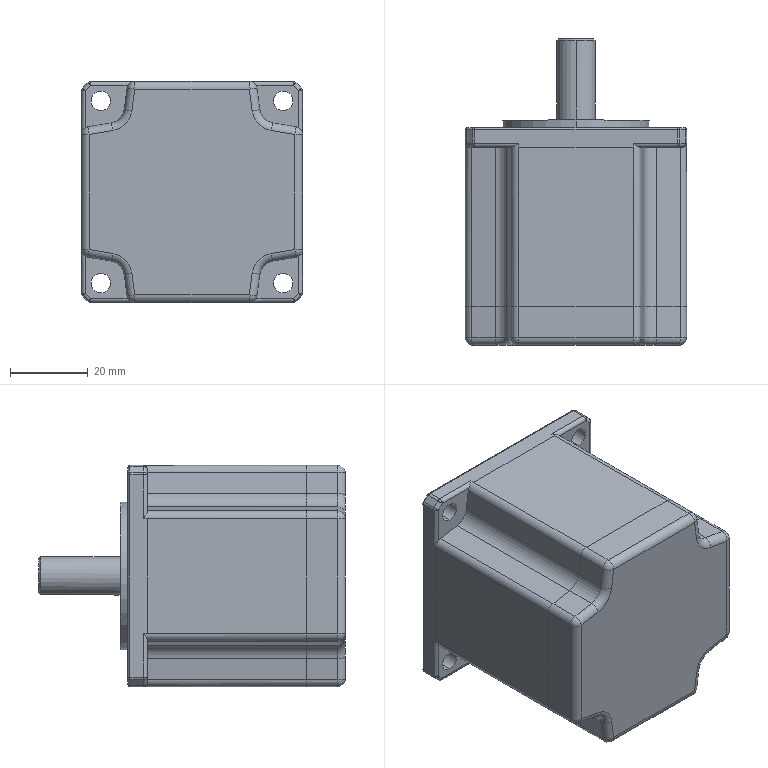Part | STEP file | 1 solid | 155 faces | box 57 x 79 x 57 mm | volume 128182 mm3 | cylinder 77 | plane 49 | sphere 16 | torus 12 | cone 1 | commonest cylinder face diameters 4 x28 2 x20 1 x8 5 x8 8 x8 10 x2